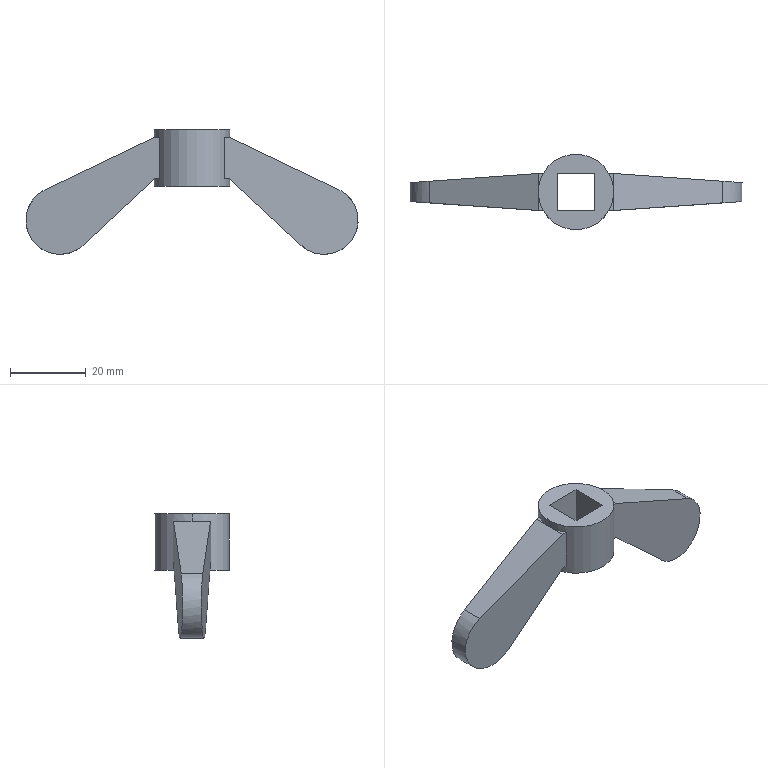Part | SolidWorks | features ICE 2, Extrusion 1, MirrorPattern 1 | 1 solid | 28 faces | box 88 x 20 x 33 mm | volume 11211 mm3 | plane 22 | cylinder 6 | commonest cylinder face diameters 18 x4 20 x2
STEP:
#1=CARTESIAN_POINT('',(35.,3.137,-25.5));
#2=VERTEX_POINT('',#1);
#3=CARTESIAN_POINT('',(28.863,3.571,-23.083));
#4=VERTEX_POINT('',#3);
#5=CARTESIAN_POINT('',(35.,3.137,-25.5));
#6=CARTESIAN_POINT('',(32.695,3.3,-25.5));
#7=CARTESIAN_POINT('',(30.55,3.452,-24.655));
#8=CARTESIAN_POINT('',(28.863,3.571,-23.083));
#9=(BOUNDED_CURVE()B_SPLINE_CURVE(3,(#5,#6,#7,#8),.UNSPECIFIED.,.F.,.T.)B_SPLINE_CURVE_WITH_KNOTS((4,4),(1.571,2.321),.UNSPECIFIED.)CURVE()GEOMETRIC_REPRESENTATION_ITEM()RATIONAL_B_SPLINE_CURVE((1.,0.9536,0.9536,1.))REPRESENTATION_ITEM(''));
#10=EDGE_CURVE('',#2,#4,#9,.T.);
#11=ORIENTED_EDGE('',*,*,#10,.F.);
#12=CARTESIAN_POINT('',(35.,-3.137,-25.5));
#13=VERTEX_POINT('',#12);
#14=CARTESIAN_POINT('',(35.,5.,-25.5));
#15=DIRECTION('',(0.,-1.,0.));
#16=VECTOR('',#15,1000.);
#17=LINE('',#14,#16);
#18=EDGE_CURVE('',#2,#13,#17,.T.);
#19=ORIENTED_EDGE('',*,*,#18,.T.);
#20=CARTESIAN_POINT('',(28.863,-3.571,-23.083));
#21=VERTEX_POINT('',#20);
#22=CARTESIAN_POINT('',(28.863,-3.571,-23.083));
#23=CARTESIAN_POINT('',(30.55,-3.452,-24.655));
#24=CARTESIAN_POINT('',(32.695,-3.3,-25.5));
#25=CARTESIAN_POINT('',(35.,-3.137,-25.5));
#26=(BOUNDED_CURVE()B_SPLINE_CURVE(3,(#22,#23,#24,#25),.UNSPECIFIED.,.F.,.T.)B_SPLINE_CURVE_WITH_KNOTS((4,4),(0.8205,1.571),.UNSPECIFIED.)CURVE()GEOMETRIC_REPRESENTATION_ITEM()RATIONAL_B_SPLINE_CURVE((1.,0.9536,0.9536,1.))REPRESENTATION_ITEM(''));
#27=EDGE_CURVE('',#21,#13,#26,.T.);
#28=ORIENTED_EDGE('',*,*,#27,.F.);
#29=CARTESIAN_POINT('',(28.863,5.,-23.083));
#30=DIRECTION('',(0.,-1.,0.));
#31=VECTOR('',#30,1000.);
#32=LINE('',#29,#31);
#33=EDGE_CURVE('',#4,#21,#32,.T.);
#34=ORIENTED_EDGE('',*,*,#33,.F.);
#35=EDGE_LOOP('',(#11,#19,#28,#34));
#36=FACE_OUTER_BOUND('',#35,.T.);
#37=CARTESIAN_POINT('',(35.,5.,-16.5));
#38=DIRECTION('',(0.,-1.,0.));
#39=DIRECTION('',(0.,0.,-1.));
#40=AXIS2_PLACEMENT_3D('',#37,#38,#39);
#41=CYLINDRICAL_SURFACE('',#40,9.);
#42=ADVANCED_FACE('',(#36),#41,.T.);
#43=CARTESIAN_POINT('',(10.,0.,7.5));
#44=VERTEX_POINT('',#43);
#45=CARTESIAN_POINT('',(-10.,0.,7.5));
#46=VERTEX_POINT('',#45);
#47=CARTESIAN_POINT('',(0.,0.,7.5));
#48=DIRECTION('',(0.,0.,1.));
#49=DIRECTION('',(1.,0.,0.));
#50=AXIS2_PLACEMENT_3D('',#47,#48,#49);
#51=CIRCLE('',#50,10.);
#52=EDGE_CURVE('',#44,#46,#51,.T.);
#53=ORIENTED_EDGE('',*,*,#52,.F.);
#54=CARTESIAN_POINT('',(10.,0.,5.5));
#55=VERTEX_POINT('',#54);
#56=CARTESIAN_POINT('',(10.,0.,7.5));
#57=DIRECTION('',(0.,0.,-1.));
#58=VECTOR('',#57,1000.);
#59=LINE('',#56,#58);
#60=EDGE_CURVE('',#44,#55,#59,.T.);
#61=ORIENTED_EDGE('',*,*,#60,.T.);
#62=CARTESIAN_POINT('',(8.66,5.,5.5));
#63=VERTEX_POINT('',#62);
#64=CARTESIAN_POINT('',(0.,0.,5.5));
#65=DIRECTION('',(0.,0.,-1.));
#66=DIRECTION('',(-1.,0.,0.));
#67=AXIS2_PLACEMENT_3D('',#64,#65,#66);
#68=CIRCLE('',#67,10.);
#69=EDGE_CURVE('',#63,#55,#68,.T.);
#70=ORIENTED_EDGE('',*,*,#69,.F.);
#71=CARTESIAN_POINT('',(8.66,5.,-5.5));
#72=VERTEX_POINT('',#71);
#73=CARTESIAN_POINT('',(8.66,5.,7.5));
#74=DIRECTION('',(0.,0.,-1.));
#75=VECTOR('',#74,1000.);
#76=LINE('',#73,#75);
#77=EDGE_CURVE('',#63,#72,#76,.T.);
#78=ORIENTED_EDGE('',*,*,#77,.T.);
#79=CARTESIAN_POINT('',(10.,0.,-5.5));
#80=VERTEX_POINT('',#79);
#81=CARTESIAN_POINT('',(0.,0.,-5.5));
#82=DIRECTION('',(0.,0.,1.));
#83=DIRECTION('',(1.,0.,0.));
#84=AXIS2_PLACEMENT_3D('',#81,#82,#83);
#85=CIRCLE('',#84,10.);
#86=EDGE_CURVE('',#80,#72,#85,.T.);
#87=ORIENTED_EDGE('',*,*,#86,.F.);
#88=CARTESIAN_POINT('',(10.,0.,-7.5));
#89=VERTEX_POINT('',#88);
#90=CARTESIAN_POINT('',(10.,0.,7.5));
#91=DIRECTION('',(0.,0.,-1.));
#92=VECTOR('',#91,1000.);
#93=LINE('',#90,#92);
#94=EDGE_CURVE('',#80,#89,#93,.T.);
#95=ORIENTED_EDGE('',*,*,#94,.T.);
#96=CARTESIAN_POINT('',(-10.,0.,-7.5));
#97=VERTEX_POINT('',#96);
#98=CARTESIAN_POINT('',(0.,0.,-7.5));
#99=DIRECTION('',(0.,0.,1.));
#100=DIRECTION('',(1.,0.,0.));
#101=AXIS2_PLACEMENT_3D('',#98,#99,#100);
#102=CIRCLE('',#101,10.);
#103=EDGE_CURVE('',#89,#97,#102,.T.);
#104=ORIENTED_EDGE('',*,*,#103,.T.);
#105=CARTESIAN_POINT('',(-10.,0.,-5.5));
#106=VERTEX_POINT('',#105);
#107=CARTESIAN_POINT('',(-10.,0.,7.5));
#108=DIRECTION('',(0.,0.,-1.));
#109=VECTOR('',#108,1000.);
#110=LINE('',#107,#109);
#111=EDGE_CURVE('',#106,#97,#110,.T.);
#112=ORIENTED_EDGE('',*,*,#111,.F.);
#113=CARTESIAN_POINT('',(-8.66,5.,-5.5));
#114=VERTEX_POINT('',#113);
#115=CARTESIAN_POINT('',(0.,0.,-5.5));
#116=DIRECTION('',(0.,0.,-1.));
#117=DIRECTION('',(-1.,0.,0.));
#118=AXIS2_PLACEMENT_3D('',#115,#116,#117);
#119=CIRCLE('',#118,10.);
#120=EDGE_CURVE('',#106,#114,#119,.T.);
#121=ORIENTED_EDGE('',*,*,#120,.T.);
#122=CARTESIAN_POINT('',(-8.66,5.,5.5));
#123=VERTEX_POINT('',#122);
#124=CARTESIAN_POINT('',(-8.66,5.,7.5));
#125=DIRECTION('',(0.,0.,1.));
#126=VECTOR('',#125,1000.);
#127=LINE('',#124,#126);
#128=EDGE_CURVE('',#114,#123,#127,.T.);
#129=ORIENTED_EDGE('',*,*,#128,.T.);
#130=CARTESIAN_POINT('',(-10.,0.,5.5));
#131=VERTEX_POINT('',#130);
#132=CARTESIAN_POINT('',(0.,0.,5.5));
#133=DIRECTION('',(0.,0.,1.));
#134=DIRECTION('',(1.,0.,0.));
#135=AXIS2_PLACEMENT_3D('',#132,#133,#134);
#136=CIRCLE('',#135,10.);
#137=EDGE_CURVE('',#123,#131,#136,.T.);
#138=ORIENTED_EDGE('',*,*,#137,.T.);
#139=CARTESIAN_POINT('',(-10.,0.,7.5));
#140=DIRECTION('',(0.,0.,-1.));
#141=VECTOR('',#140,1000.);
#142=LINE('',#139,#141);
#143=EDGE_CURVE('',#46,#131,#142,.T.);
#144=ORIENTED_EDGE('',*,*,#143,.F.);
#145=EDGE_LOOP('',(#53,#61,#70,#78,#87,#95,#104,#112,#121,#129,#138,#144));
#146=FACE_OUTER_BOUND('',#145,.T.);
#147=CARTESIAN_POINT('',(0.,0.,7.5));
#148=DIRECTION('',(0.,0.,-1.));
#149=DIRECTION('',(-1.,0.,0.));
#150=AXIS2_PLACEMENT_3D('',#147,#148,#149);
#151=CYLINDRICAL_SURFACE('',#150,10.);
#152=ADVANCED_FACE('',(#146),#151,.T.);
#153=CARTESIAN_POINT('',(-35.,3.137,-25.5));
#154=VERTEX_POINT('',#153);
#155=CARTESIAN_POINT('',(-38.898,2.861,-8.388));
#156=VERTEX_POINT('',#155);
#157=CARTESIAN_POINT('',(-35.,3.137,-25.5));
#158=CARTESIAN_POINT('',(-47.152,2.277,-25.5));
#159=CARTESIAN_POINT('',(-49.851,2.086,-13.652));
#160=CARTESIAN_POINT('',(-38.898,2.861,-8.388));
#161=(BOUNDED_CURVE()B_SPLINE_CURVE(3,(#157,#158,#159,#160),.UNSPECIFIED.,.F.,.T.)B_SPLINE_CURVE_WITH_KNOTS((4,4),(4.712,7.406),.UNSPECIFIED.)CURVE()GEOMETRIC_REPRESENTATION_ITEM()RATIONAL_B_SPLINE_CURVE((1.,0.4814,0.4814,1.))REPRESENTATION_ITEM(''));
#162=EDGE_CURVE('',#154,#156,#161,.T.);
#163=ORIENTED_EDGE('',*,*,#162,.F.);
#164=CARTESIAN_POINT('',(-35.,-3.137,-25.5));
#165=VERTEX_POINT('',#164);
#166=CARTESIAN_POINT('',(-35.,5.,-25.5));
#167=DIRECTION('',(0.,-1.,0.));
#168=VECTOR('',#167,1000.);
#169=LINE('',#166,#168);
#170=EDGE_CURVE('',#154,#165,#169,.T.);
#171=ORIENTED_EDGE('',*,*,#170,.T.);
#172=CARTESIAN_POINT('',(-38.898,-2.861,-8.388));
#173=VERTEX_POINT('',#172);
#174=CARTESIAN_POINT('',(-38.898,-2.861,-8.388));
#175=CARTESIAN_POINT('',(-49.851,-2.086,-13.652));
#176=CARTESIAN_POINT('',(-47.152,-2.277,-25.5));
#177=CARTESIAN_POINT('',(-35.,-3.137,-25.5));
#178=(BOUNDED_CURVE()B_SPLINE_CURVE(3,(#174,#175,#176,#177),.UNSPECIFIED.,.F.,.T.)B_SPLINE_CURVE_WITH_KNOTS((4,4),(2.019,4.712),.UNSPECIFIED.)CURVE()GEOMETRIC_REPRESENTATION_ITEM()RATIONAL_B_SPLINE_CURVE((1.,0.4814,0.4814,1.))REPRESENTATION_ITEM(''));
#179=EDGE_CURVE('',#173,#165,#178,.T.);
#180=ORIENTED_EDGE('',*,*,#179,.F.);
#181=CARTESIAN_POINT('',(-38.898,5.,-8.388));
#182=DIRECTION('',(0.,-1.,0.));
#183=VECTOR('',#182,1000.);
#184=LINE('',#181,#183);
#185=EDGE_CURVE('',#156,#173,#184,.T.);
#186=ORIENTED_EDGE('',*,*,#185,.F.);
#187=EDGE_LOOP('',(#163,#171,#180,#186));
#188=FACE_OUTER_BOUND('',#187,.T.);
#189=CARTESIAN_POINT('',(-35.,5.,-16.5));
#190=DIRECTION('',(0.,-1.,0.));
#191=DIRECTION('',(0.,0.,-1.));
#192=AXIS2_PLACEMENT_3D('',#189,#190,#191);
#193=CYLINDRICAL_SURFACE('',#192,9.);
#194=ADVANCED_FACE('',(#188),#193,.T.);
#195=CARTESIAN_POINT('',(-10.,-4.905,-5.5));
#196=VERTEX_POINT('',#195);
#197=CARTESIAN_POINT('',(-10.,5.,-5.5));
#198=DIRECTION('',(0.,-1.,0.));
#199=VECTOR('',#198,1000.);
#200=LINE('',#197,#199);
#201=EDGE_CURVE('',#106,#196,#200,.T.);
#202=ORIENTED_EDGE('',*,*,#201,.T.);
#203=CARTESIAN_POINT('',(-28.863,-3.571,-23.083));
#204=VERTEX_POINT('',#203);
#205=CARTESIAN_POINT('',(-2.302,-5.45,1.676));
#206=DIRECTION('',(-0.7305,0.05168,-0.6809));
#207=VECTOR('',#206,1000.);
#208=LINE('',#205,#207);
#209=EDGE_CURVE('',#196,#204,#208,.T.);
#210=ORIENTED_EDGE('',*,*,#209,.T.);
#211=CARTESIAN_POINT('',(-28.863,3.571,-23.083));
#212=VERTEX_POINT('',#211);
#213=CARTESIAN_POINT('',(-28.863,5.,-23.083));
#214=DIRECTION('',(0.,-1.,0.));
#215=VECTOR('',#214,1000.);
#216=LINE('',#213,#215);
#217=EDGE_CURVE('',#212,#204,#216,.T.);
#218=ORIENTED_EDGE('',*,*,#217,.F.);
#219=CARTESIAN_POINT('',(-10.,4.905,-5.5));
#220=VERTEX_POINT('',#219);
#221=CARTESIAN_POINT('',(-1.924,5.477,2.028));
#222=DIRECTION('',(0.7305,0.05168,0.6809));
#223=VECTOR('',#222,1000.);
#224=LINE('',#221,#223);
#225=EDGE_CURVE('',#212,#220,#224,.T.);
#226=ORIENTED_EDGE('',*,*,#225,.T.);
#227=CARTESIAN_POINT('',(-10.,5.,-5.5));
#228=DIRECTION('',(0.,-1.,0.));
#229=VECTOR('',#228,1000.);
#230=LINE('',#227,#229);
#231=EDGE_CURVE('',#220,#106,#230,.T.);
#232=ORIENTED_EDGE('',*,*,#231,.T.);
#233=EDGE_LOOP('',(#202,#210,#218,#226,#232));
#234=FACE_OUTER_BOUND('',#233,.T.);
#235=CARTESIAN_POINT('',(-1.906,5.,2.045));
#236=DIRECTION('',(0.6819,0.,-0.7315));
#237=DIRECTION('',(-0.7315,0.,-0.6819));
#238=AXIS2_PLACEMENT_3D('',#235,#236,#237);
#239=PLANE('',#238);
#240=ADVANCED_FACE('',(#234),#239,.T.);
#241=ORIENTED_EDGE('',*,*,#170,.F.);
#242=CARTESIAN_POINT('',(-28.863,3.571,-23.083));
#243=CARTESIAN_POINT('',(-30.55,3.452,-24.655));
#244=CARTESIAN_POINT('',(-32.695,3.3,-25.5));
#245=CARTESIAN_POINT('',(-35.,3.137,-25.5));
#246=(BOUNDED_CURVE()B_SPLINE_CURVE(3,(#242,#243,#244,#245),.UNSPECIFIED.,.F.,.T.)B_SPLINE_CURVE_WITH_KNOTS((4,4),(3.962,4.712),.UNSPECIFIED.)CURVE()GEOMETRIC_REPRESENTATION_ITEM()RATIONAL_B_SPLINE_CURVE((1.,0.9536,0.9536,1.))REPRESENTATION_ITEM(''));
#247=EDGE_CURVE('',#212,#154,#246,.T.);
#248=ORIENTED_EDGE('',*,*,#247,.F.);
#249=ORIENTED_EDGE('',*,*,#217,.T.);
#250=CARTESIAN_POINT('',(-35.,-3.137,-25.5));
#251=CARTESIAN_POINT('',(-32.695,-3.3,-25.5));
#252=CARTESIAN_POINT('',(-30.55,-3.452,-24.655));
#253=CARTESIAN_POINT('',(-28.863,-3.571,-23.083));
#254=(BOUNDED_CURVE()B_SPLINE_CURVE(3,(#250,#251,#252,#253),.UNSPECIFIED.,.F.,.F.)B_SPLINE_CURVE_WITH_KNOTS((4,4),(4.712,5.463),.UNSPECIFIED.)CURVE()GEOMETRIC_REPRESENTATION_ITEM()RATIONAL_B_SPLINE_CURVE((1.,0.9536,0.9536,1.))REPRESENTATION_ITEM(''));
#255=EDGE_CURVE('',#165,#204,#254,.T.);
#256=ORIENTED_EDGE('',*,*,#255,.F.);
#257=EDGE_LOOP('',(#241,#248,#249,#256));
#258=FACE_OUTER_BOUND('',#257,.T.);
#259=CARTESIAN_POINT('',(-35.,5.,-16.5));
#260=DIRECTION('',(0.,-1.,0.));
#261=DIRECTION('',(0.,0.,-1.));
#262=AXIS2_PLACEMENT_3D('',#259,#260,#261);
#263=CYLINDRICAL_SURFACE('',#262,9.);
#264=ADVANCED_FACE('',(#258),#263,.T.);
#265=CARTESIAN_POINT('',(-10.,-4.905,5.5));
#266=VERTEX_POINT('',#265);
#267=CARTESIAN_POINT('',(-4.615,-5.286,8.088));
#268=DIRECTION('',(-0.8995,0.06363,-0.4323));
#269=VECTOR('',#268,1000.);
#270=LINE('',#267,#269);
#271=EDGE_CURVE('',#266,#173,#270,.T.);
#272=ORIENTED_EDGE('',*,*,#271,.F.);
#273=CARTESIAN_POINT('',(-10.,5.,5.5));
#274=DIRECTION('',(0.,-1.,0.));
#275=VECTOR('',#274,1000.);
#276=LINE('',#273,#275);
#277=EDGE_CURVE('',#131,#266,#276,.T.);
#278=ORIENTED_EDGE('',*,*,#277,.F.);
#279=CARTESIAN_POINT('',(-10.,4.905,5.5));
#280=VERTEX_POINT('',#279);
#281=CARTESIAN_POINT('',(-10.,5.,5.5));
#282=DIRECTION('',(0.,-1.,0.));
#283=VECTOR('',#282,1000.);
#284=LINE('',#281,#283);
#285=EDGE_CURVE('',#280,#131,#284,.T.);
#286=ORIENTED_EDGE('',*,*,#285,.F.);
#287=CARTESIAN_POINT('',(-4.042,5.327,8.363));
#288=DIRECTION('',(0.8995,0.06363,0.4323));
#289=VECTOR('',#288,1000.);
#290=LINE('',#287,#289);
#291=EDGE_CURVE('',#156,#280,#290,.T.);
#292=ORIENTED_EDGE('',*,*,#291,.F.);
#293=ORIENTED_EDGE('',*,*,#185,.T.);
#294=EDGE_LOOP('',(#272,#278,#286,#292,#293));
#295=FACE_OUTER_BOUND('',#294,.T.);
#296=CARTESIAN_POINT('',(-4.024,5.,8.372));
#297=DIRECTION('',(0.4332,0.,-0.9013));
#298=DIRECTION('',(-0.9013,0.,-0.4332));
#299=AXIS2_PLACEMENT_3D('',#296,#297,#298);
#300=PLANE('',#299);
#301=ADVANCED_FACE('',(#295),#300,.F.);
#302=ORIENTED_EDGE('',*,*,#277,.T.);
#303=CARTESIAN_POINT('',(-8.66,-5.,5.5));
#304=VERTEX_POINT('',#303);
#305=CARTESIAN_POINT('',(-0.747,-5.56,5.5));
#306=DIRECTION('',(0.9975,-0.07057,0.));
#307=VECTOR('',#306,1000.);
#308=LINE('',#305,#307);
#309=EDGE_CURVE('',#266,#304,#308,.T.);
#310=ORIENTED_EDGE('',*,*,#309,.T.);
#311=CARTESIAN_POINT('',(0.,0.,5.5));
#312=DIRECTION('',(0.,0.,1.));
#313=DIRECTION('',(1.,0.,0.));
#314=AXIS2_PLACEMENT_3D('',#311,#312,#313);
#315=CIRCLE('',#314,10.);
#316=EDGE_CURVE('',#131,#304,#315,.T.);
#317=ORIENTED_EDGE('',*,*,#316,.F.);
#318=EDGE_LOOP('',(#302,#310,#317));
#319=FACE_OUTER_BOUND('',#318,.T.);
#320=CARTESIAN_POINT('',(0.,5.,5.5));
#321=DIRECTION('',(0.,0.,1.));
#322=DIRECTION('',(1.,0.,0.));
#323=AXIS2_PLACEMENT_3D('',#320,#321,#322);
#324=PLANE('',#323);
#325=ADVANCED_FACE('',(#319),#324,.T.);
#326=CARTESIAN_POINT('',(-8.66,-5.,-5.5));
#327=VERTEX_POINT('',#326);
#328=CARTESIAN_POINT('',(0.,0.,-5.5));
#329=DIRECTION('',(0.,0.,-1.));
#330=DIRECTION('',(-1.,0.,0.));
#331=AXIS2_PLACEMENT_3D('',#328,#329,#330);
#332=CIRCLE('',#331,10.);
#333=EDGE_CURVE('',#327,#106,#332,.T.);
#334=ORIENTED_EDGE('',*,*,#333,.F.);
#335=CARTESIAN_POINT('',(-0.747,-5.56,-5.5));
#336=DIRECTION('',(-0.9975,0.07057,0.));
#337=VECTOR('',#336,1000.);
#338=LINE('',#335,#337);
#339=EDGE_CURVE('',#327,#196,#338,.T.);
#340=ORIENTED_EDGE('',*,*,#339,.T.);
#341=ORIENTED_EDGE('',*,*,#201,.F.);
#342=EDGE_LOOP('',(#334,#340,#341));
#343=FACE_OUTER_BOUND('',#342,.T.);
#344=CARTESIAN_POINT('',(0.,5.,-5.5));
#345=DIRECTION('',(0.,0.,-1.));
#346=DIRECTION('',(-1.,0.,0.));
#347=AXIS2_PLACEMENT_3D('',#344,#345,#346);
#348=PLANE('',#347);
#349=ADVANCED_FACE('',(#343),#348,.T.);
#350=ORIENTED_EDGE('',*,*,#137,.F.);
#351=CARTESIAN_POINT('',(-0.04312,5.61,5.5));
#352=DIRECTION('',(-0.9975,-0.07057,0.));
#353=VECTOR('',#352,1000.);
#354=LINE('',#351,#353);
#355=EDGE_CURVE('',#123,#280,#354,.T.);
#356=ORIENTED_EDGE('',*,*,#355,.T.);
#357=ORIENTED_EDGE('',*,*,#285,.T.);
#358=EDGE_LOOP('',(#350,#356,#357));
#359=FACE_OUTER_BOUND('',#358,.T.);
#360=CARTESIAN_POINT('',(0.,5.,5.5));
#361=DIRECTION('',(0.,0.,1.));
#362=DIRECTION('',(1.,0.,0.));
#363=AXIS2_PLACEMENT_3D('',#360,#361,#362);
#364=PLANE('',#363);
#365=ADVANCED_FACE('',(#359),#364,.T.);
#366=ORIENTED_EDGE('',*,*,#231,.F.);
#367=CARTESIAN_POINT('',(-0.04312,5.61,-5.5));
#368=DIRECTION('',(0.9975,0.07057,0.));
#369=VECTOR('',#368,1000.);
#370=LINE('',#367,#369);
#371=EDGE_CURVE('',#220,#114,#370,.T.);
#372=ORIENTED_EDGE('',*,*,#371,.T.);
#373=ORIENTED_EDGE('',*,*,#120,.F.);
#374=EDGE_LOOP('',(#366,#372,#373));
#375=FACE_OUTER_BOUND('',#374,.T.);
#376=CARTESIAN_POINT('',(0.,5.,-5.5));
#377=DIRECTION('',(0.,0.,-1.));
#378=DIRECTION('',(-1.,0.,0.));
#379=AXIS2_PLACEMENT_3D('',#376,#377,#378);
#380=PLANE('',#379);
#381=ADVANCED_FACE('',(#375),#380,.T.);
#382=CARTESIAN_POINT('',(0.,0.,7.5));
#383=DIRECTION('',(0.,0.,1.));
#384=DIRECTION('',(1.,0.,0.));
#385=AXIS2_PLACEMENT_3D('',#382,#383,#384);
#386=CIRCLE('',#385,10.);
#387=EDGE_CURVE('',#46,#44,#386,.T.);
#388=ORIENTED_EDGE('',*,*,#387,.T.);
#389=ORIENTED_EDGE('',*,*,#52,.T.);
#390=EDGE_LOOP('',(#388,#389));
#391=FACE_OUTER_BOUND('',#390,.T.);
#392=CARTESIAN_POINT('',(5.,5.,7.5));
#393=VERTEX_POINT('',#392);
#394=CARTESIAN_POINT('',(-5.,5.,7.5));
#395=VERTEX_POINT('',#394);
#396=CARTESIAN_POINT('',(-5.,5.,7.5));
#397=DIRECTION('',(-1.,0.,0.));
#398=VECTOR('',#397,1000.);
#399=LINE('',#396,#398);
#400=EDGE_CURVE('',#393,#395,#399,.T.);
#401=ORIENTED_EDGE('',*,*,#400,.F.);
#402=CARTESIAN_POINT('',(5.,-5.,7.5));
#403=VERTEX_POINT('',#402);
#404=CARTESIAN_POINT('',(5.,-5.,7.5));
#405=DIRECTION('',(0.,1.,0.));
#406=VECTOR('',#405,1000.);
#407=LINE('',#404,#406);
#408=EDGE_CURVE('',#403,#393,#407,.T.);
#409=ORIENTED_EDGE('',*,*,#408,.F.);
#410=CARTESIAN_POINT('',(-5.,-5.,7.5));
#411=VERTEX_POINT('',#410);
#412=CARTESIAN_POINT('',(-5.,-5.,7.5));
#413=DIRECTION('',(1.,0.,0.));
#414=VECTOR('',#413,1000.);
#415=LINE('',#412,#414);
#416=EDGE_CURVE('',#411,#403,#415,.T.);
#417=ORIENTED_EDGE('',*,*,#416,.F.);
#418=CARTESIAN_POINT('',(-5.,-5.,7.5));
#419=DIRECTION('',(0.,-1.,0.));
#420=VECTOR('',#419,1000.);
#421=LINE('',#418,#420);
#422=EDGE_CURVE('',#395,#411,#421,.T.);
#423=ORIENTED_EDGE('',*,*,#422,.F.);
#424=EDGE_LOOP('',(#401,#409,#417,#423));
#425=FACE_BOUND('',#424,.T.);
#426=CARTESIAN_POINT('',(0.,0.,7.5));
#427=DIRECTION('',(0.,0.,1.));
#428=DIRECTION('',(1.,0.,0.));
#429=AXIS2_PLACEMENT_3D('',#426,#427,#428);
#430=PLANE('',#429);
#431=ADVANCED_FACE('',(#391,#425),#430,.T.);
#432=CARTESIAN_POINT('',(0.,0.,-7.5));
#433=DIRECTION('',(0.,0.,1.));
#434=DIRECTION('',(1.,0.,0.));
#435=AXIS2_PLACEMENT_3D('',#432,#433,#434);
#436=CIRCLE('',#435,10.);
#437=EDGE_CURVE('',#97,#89,#436,.T.);
#438=ORIENTED_EDGE('',*,*,#437,.F.);
#439=ORIENTED_EDGE('',*,*,#103,.F.);
#440=EDGE_LOOP('',(#438,#439));
#441=FACE_OUTER_BOUND('',#440,.T.);
#442=CARTESIAN_POINT('',(5.,-5.,-7.5));
#443=VERTEX_POINT('',#442);
#444=CARTESIAN_POINT('',(5.,5.,-7.5));
#445=VERTEX_POINT('',#444);
#446=CARTESIAN_POINT('',(5.,-5.,-7.5));
#447=DIRECTION('',(0.,1.,0.));
#448=VECTOR('',#447,1000.);
#449=LINE('',#446,#448);
#450=EDGE_CURVE('',#443,#445,#449,.T.);
#451=ORIENTED_EDGE('',*,*,#450,.T.);
#452=CARTESIAN_POINT('',(-5.,5.,-7.5));
#453=VERTEX_POINT('',#452);
#454=CARTESIAN_POINT('',(-5.,5.,-7.5));
#455=DIRECTION('',(-1.,0.,0.));
#456=VECTOR('',#455,1000.);
#457=LINE('',#454,#456);
#458=EDGE_CURVE('',#445,#453,#457,.T.);
#459=ORIENTED_EDGE('',*,*,#458,.T.);
#460=CARTESIAN_POINT('',(-5.,-5.,-7.5));
#461=VERTEX_POINT('',#460);
#462=CARTESIAN_POINT('',(-5.,-5.,-7.5));
#463=DIRECTION('',(0.,-1.,0.));
#464=VECTOR('',#463,1000.);
#465=LINE('',#462,#464);
#466=EDGE_CURVE('',#453,#461,#465,.T.);
#467=ORIENTED_EDGE('',*,*,#466,.T.);
#468=CARTESIAN_POINT('',(-5.,-5.,-7.5));
#469=DIRECTION('',(1.,0.,0.));
#470=VECTOR('',#469,1000.);
#471=LINE('',#468,#470);
#472=EDGE_CURVE('',#461,#443,#471,.T.);
#473=ORIENTED_EDGE('',*,*,#472,.T.);
#474=EDGE_LOOP('',(#451,#459,#467,#473));
#475=FACE_BOUND('',#474,.T.);
#476=CARTESIAN_POINT('',(0.,0.,-7.5));
#477=DIRECTION('',(0.,0.,1.));
#478=DIRECTION('',(1.,0.,0.));
#479=AXIS2_PLACEMENT_3D('',#476,#477,#478);
#480=PLANE('',#479);
#481=ADVANCED_FACE('',(#441,#475),#480,.F.);
#482=ORIENTED_EDGE('',*,*,#60,.F.);
#483=ORIENTED_EDGE('',*,*,#387,.F.);
#484=ORIENTED_EDGE('',*,*,#143,.T.);
#485=ORIENTED_EDGE('',*,*,#316,.T.);
#486=CARTESIAN_POINT('',(-8.66,-5.,7.5));
#487=DIRECTION('',(0.,0.,1.));
#488=VECTOR('',#487,1000.);
#489=LINE('',#486,#488);
#490=EDGE_CURVE('',#327,#304,#489,.T.);
#491=ORIENTED_EDGE('',*,*,#490,.F.);
#492=ORIENTED_EDGE('',*,*,#333,.T.);
#493=ORIENTED_EDGE('',*,*,#111,.T.);
#494=ORIENTED_EDGE('',*,*,#437,.T.);
#495=ORIENTED_EDGE('',*,*,#94,.F.);
#496=CARTESIAN_POINT('',(8.66,-5.,-5.5));
#497=VERTEX_POINT('',#496);
#498=CARTESIAN_POINT('',(0.,0.,-5.5));
#499=DIRECTION('',(0.,0.,1.));
#500=DIRECTION('',(1.,0.,0.));
#501=AXIS2_PLACEMENT_3D('',#498,#499,#500);
#502=CIRCLE('',#501,10.);
#503=EDGE_CURVE('',#497,#80,#502,.T.);
#504=ORIENTED_EDGE('',*,*,#503,.F.);
#505=CARTESIAN_POINT('',(8.66,-5.,5.5));
#506=VERTEX_POINT('',#505);
#507=CARTESIAN_POINT('',(8.66,-5.,7.5));
#508=DIRECTION('',(0.,0.,-1.));
#509=VECTOR('',#508,1000.);
#510=LINE('',#507,#509);
#511=EDGE_CURVE('',#506,#497,#510,.T.);
#512=ORIENTED_EDGE('',*,*,#511,.F.);
#513=CARTESIAN_POINT('',(0.,0.,5.5));
#514=DIRECTION('',(0.,0.,-1.));
#515=DIRECTION('',(-1.,0.,0.));
#516=AXIS2_PLACEMENT_3D('',#513,#514,#515);
#517=CIRCLE('',#516,10.);
#518=EDGE_CURVE('',#55,#506,#517,.T.);
#519=ORIENTED_EDGE('',*,*,#518,.F.);
#520=EDGE_LOOP('',(#482,#483,#484,#485,#491,#492,#493,#494,#495,#504,#512,#519));
#521=FACE_OUTER_BOUND('',#520,.T.);
#522=CARTESIAN_POINT('',(0.,0.,7.5));
#523=DIRECTION('',(0.,0.,-1.));
#524=DIRECTION('',(-1.,0.,0.));
#525=AXIS2_PLACEMENT_3D('',#522,#523,#524);
#526=CYLINDRICAL_SURFACE('',#525,10.);
#527=ADVANCED_FACE('',(#521),#526,.T.);
#528=ORIENTED_EDGE('',*,*,#450,.F.);
#529=CARTESIAN_POINT('',(5.,-5.,7.5));
#530=DIRECTION('',(0.,0.,-1.));
#531=VECTOR('',#530,1000.);
#532=LINE('',#529,#531);
#533=EDGE_CURVE('',#403,#443,#532,.T.);
#534=ORIENTED_EDGE('',*,*,#533,.F.);
#535=ORIENTED_EDGE('',*,*,#408,.T.);
#536=CARTESIAN_POINT('',(5.,5.,7.5));
#537=DIRECTION('',(0.,0.,-1.));
#538=VECTOR('',#537,1000.);
#539=LINE('',#536,#538);
#540=EDGE_CURVE('',#393,#445,#539,.T.);
#541=ORIENTED_EDGE('',*,*,#540,.T.);
#542=EDGE_LOOP('',(#528,#534,#535,#541));
#543=FACE_OUTER_BOUND('',#542,.T.);
#544=CARTESIAN_POINT('',(5.,-5.,7.5));
#545=DIRECTION('',(-1.,0.,0.));
#546=DIRECTION('',(0.,0.,1.));
#547=AXIS2_PLACEMENT_3D('',#544,#545,#546);
#548=PLANE('',#547);
#549=ADVANCED_FACE('',(#543),#548,.T.);
#550=ORIENTED_EDGE('',*,*,#458,.F.);
#551=ORIENTED_EDGE('',*,*,#540,.F.);
#552=ORIENTED_EDGE('',*,*,#400,.T.);
#553=CARTESIAN_POINT('',(-5.,5.,7.5));
#554=DIRECTION('',(0.,0.,-1.));
#555=VECTOR('',#554,1000.);
#556=LINE('',#553,#555);
#557=EDGE_CURVE('',#395,#453,#556,.T.);
#558=ORIENTED_EDGE('',*,*,#557,.T.);
#559=EDGE_LOOP('',(#550,#551,#552,#558));
#560=FACE_OUTER_BOUND('',#559,.T.);
#561=CARTESIAN_POINT('',(-5.,5.,7.5));
#562=DIRECTION('',(0.,-1.,0.));
#563=DIRECTION('',(0.,0.,-1.));
#564=AXIS2_PLACEMENT_3D('',#561,#562,#563);
#565=PLANE('',#564);
#566=ADVANCED_FACE('',(#560),#565,.T.);
#567=ORIENTED_EDGE('',*,*,#466,.F.);
#568=ORIENTED_EDGE('',*,*,#557,.F.);
#569=ORIENTED_EDGE('',*,*,#422,.T.);
#570=CARTESIAN_POINT('',(-5.,-5.,7.5));
#571=DIRECTION('',(0.,0.,-1.));
#572=VECTOR('',#571,1000.);
#573=LINE('',#570,#572);
#574=EDGE_CURVE('',#411,#461,#573,.T.);
#575=ORIENTED_EDGE('',*,*,#574,.T.);
#576=EDGE_LOOP('',(#567,#568,#569,#575));
#577=FACE_OUTER_BOUND('',#576,.T.);
#578=CARTESIAN_POINT('',(-5.,-5.,7.5));
#579=DIRECTION('',(1.,0.,0.));
#580=DIRECTION('',(0.,0.,-1.));
#581=AXIS2_PLACEMENT_3D('',#578,#579,#580);
#582=PLANE('',#581);
#583=ADVANCED_FACE('',(#577),#582,.T.);
#584=ORIENTED_EDGE('',*,*,#472,.F.);
#585=ORIENTED_EDGE('',*,*,#574,.F.);
#586=ORIENTED_EDGE('',*,*,#416,.T.);
#587=ORIENTED_EDGE('',*,*,#533,.T.);
#588=EDGE_LOOP('',(#584,#585,#586,#587));
#589=FACE_OUTER_BOUND('',#588,.T.);
#590=CARTESIAN_POINT('',(-5.,-5.,7.5));
#591=DIRECTION('',(0.,1.,0.));
#592=DIRECTION('',(0.,0.,1.));
#593=AXIS2_PLACEMENT_3D('',#590,#591,#592);
#594=PLANE('',#593);
#595=ADVANCED_FACE('',(#589),#594,.T.);
#596=ORIENTED_EDGE('',*,*,#225,.F.);
#597=ORIENTED_EDGE('',*,*,#247,.T.);
#598=ORIENTED_EDGE('',*,*,#162,.T.);
#599=ORIENTED_EDGE('',*,*,#291,.T.);
#600=ORIENTED_EDGE('',*,*,#355,.F.);
#601=ORIENTED_EDGE('',*,*,#128,.F.);
#602=ORIENTED_EDGE('',*,*,#371,.F.);
#603=EDGE_LOOP('',(#596,#597,#598,#599,#600,#601,#602));
#604=FACE_OUTER_BOUND('',#603,.T.);
#605=CARTESIAN_POINT('',(-0.3951,5.585,-38.));
#606=DIRECTION('',(-0.07057,0.9975,0.));
#607=DIRECTION('',(-0.9975,-0.07057,0.));
#608=AXIS2_PLACEMENT_3D('',#605,#606,#607);
#609=PLANE('',#608);
#610=ADVANCED_FACE('',(#604),#609,.T.);
#611=ORIENTED_EDGE('',*,*,#271,.T.);
#612=ORIENTED_EDGE('',*,*,#179,.T.);
#613=ORIENTED_EDGE('',*,*,#255,.T.);
#614=ORIENTED_EDGE('',*,*,#209,.F.);
#615=ORIENTED_EDGE('',*,*,#339,.F.);
#616=ORIENTED_EDGE('',*,*,#490,.T.);
#617=ORIENTED_EDGE('',*,*,#309,.F.);
#618=EDGE_LOOP('',(#611,#612,#613,#614,#615,#616,#617));
#619=FACE_OUTER_BOUND('',#618,.T.);
#620=CARTESIAN_POINT('',(-0.3951,-5.585,-38.));
#621=DIRECTION('',(-0.07057,-0.9975,0.));
#622=DIRECTION('',(0.9975,-0.07057,0.));
#623=AXIS2_PLACEMENT_3D('',#620,#621,#622);
#624=PLANE('',#623);
#625=ADVANCED_FACE('',(#619),#624,.T.);
#626=ORIENTED_EDGE('',*,*,#86,.T.);
#627=CARTESIAN_POINT('',(10.,4.905,-5.5));
#628=VERTEX_POINT('',#627);
#629=CARTESIAN_POINT('',(0.04312,5.61,-5.5));
#630=DIRECTION('',(0.9975,-0.07057,0.));
#631=VECTOR('',#630,1000.);
#632=LINE('',#629,#631);
#633=EDGE_CURVE('',#72,#628,#632,.T.);
#634=ORIENTED_EDGE('',*,*,#633,.T.);
#635=CARTESIAN_POINT('',(10.,5.,-5.5));
#636=DIRECTION('',(0.,-1.,0.));
#637=VECTOR('',#636,1000.);
#638=LINE('',#635,#637);
#639=EDGE_CURVE('',#628,#80,#638,.T.);
#640=ORIENTED_EDGE('',*,*,#639,.T.);
#641=EDGE_LOOP('',(#626,#634,#640));
#642=FACE_OUTER_BOUND('',#641,.T.);
#643=CARTESIAN_POINT('',(0.,5.,-5.5));
#644=DIRECTION('',(0.,0.,1.));
#645=DIRECTION('',(1.,0.,0.));
#646=AXIS2_PLACEMENT_3D('',#643,#644,#645);
#647=PLANE('',#646);
#648=ADVANCED_FACE('',(#642),#647,.F.);
#649=CARTESIAN_POINT('',(10.,-4.905,-5.5));
#650=VERTEX_POINT('',#649);
#651=CARTESIAN_POINT('',(10.,5.,-5.5));
#652=DIRECTION('',(0.,-1.,0.));
#653=VECTOR('',#652,1000.);
#654=LINE('',#651,#653);
#655=EDGE_CURVE('',#80,#650,#654,.T.);
#656=ORIENTED_EDGE('',*,*,#655,.T.);
#657=CARTESIAN_POINT('',(0.747,-5.56,-5.5));
#658=DIRECTION('',(-0.9975,-0.07057,0.));
#659=VECTOR('',#658,1000.);
#660=LINE('',#657,#659);
#661=EDGE_CURVE('',#650,#497,#660,.T.);
#662=ORIENTED_EDGE('',*,*,#661,.T.);
#663=ORIENTED_EDGE('',*,*,#503,.T.);
#664=EDGE_LOOP('',(#656,#662,#663));
#665=FACE_OUTER_BOUND('',#664,.T.);
#666=CARTESIAN_POINT('',(0.,5.,-5.5));
#667=DIRECTION('',(0.,0.,1.));
#668=DIRECTION('',(1.,0.,0.));
#669=AXIS2_PLACEMENT_3D('',#666,#667,#668);
#670=PLANE('',#669);
#671=ADVANCED_FACE('',(#665),#670,.F.);
#672=CARTESIAN_POINT('',(10.,4.905,5.5));
#673=VERTEX_POINT('',#672);
#674=CARTESIAN_POINT('',(10.,5.,5.5));
#675=DIRECTION('',(0.,-1.,0.));
#676=VECTOR('',#675,1000.);
#677=LINE('',#674,#676);
#678=EDGE_CURVE('',#673,#55,#677,.T.);
#679=ORIENTED_EDGE('',*,*,#678,.F.);
#680=CARTESIAN_POINT('',(0.04312,5.61,5.5));
#681=DIRECTION('',(-0.9975,0.07057,0.));
#682=VECTOR('',#681,1000.);
#683=LINE('',#680,#682);
#684=EDGE_CURVE('',#673,#63,#683,.T.);
#685=ORIENTED_EDGE('',*,*,#684,.T.);
#686=ORIENTED_EDGE('',*,*,#69,.T.);
#687=EDGE_LOOP('',(#679,#685,#686));
#688=FACE_OUTER_BOUND('',#687,.T.);
#689=CARTESIAN_POINT('',(0.,5.,5.5));
#690=DIRECTION('',(0.,0.,-1.));
#691=DIRECTION('',(-1.,0.,0.));
#692=AXIS2_PLACEMENT_3D('',#689,#690,#691);
#693=PLANE('',#692);
#694=ADVANCED_FACE('',(#688),#693,.F.);
#695=ORIENTED_EDGE('',*,*,#518,.T.);
#696=CARTESIAN_POINT('',(10.,-4.905,5.5));
#697=VERTEX_POINT('',#696);
#698=CARTESIAN_POINT('',(0.747,-5.56,5.5));
#699=DIRECTION('',(0.9975,0.07057,0.));
#700=VECTOR('',#699,1000.);
#701=LINE('',#698,#700);
#702=EDGE_CURVE('',#506,#697,#701,.T.);
#703=ORIENTED_EDGE('',*,*,#702,.T.);
#704=CARTESIAN_POINT('',(10.,5.,5.5));
#705=DIRECTION('',(0.,-1.,0.));
#706=VECTOR('',#705,1000.);
#707=LINE('',#704,#706);
#708=EDGE_CURVE('',#55,#697,#707,.T.);
#709=ORIENTED_EDGE('',*,*,#708,.F.);
#710=EDGE_LOOP('',(#695,#703,#709));
#711=FACE_OUTER_BOUND('',#710,.T.);
#712=CARTESIAN_POINT('',(0.,5.,5.5));
#713=DIRECTION('',(0.,0.,-1.));
#714=DIRECTION('',(-1.,0.,0.));
#715=AXIS2_PLACEMENT_3D('',#712,#713,#714);
#716=PLANE('',#715);
#717=ADVANCED_FACE('',(#711),#716,.F.);
#718=ORIENTED_EDGE('',*,*,#33,.T.);
#719=CARTESIAN_POINT('',(2.302,-5.45,1.676));
#720=DIRECTION('',(-0.7305,-0.05168,0.6809));
#721=VECTOR('',#720,1000.);
#722=LINE('',#719,#721);
#723=EDGE_CURVE('',#21,#650,#722,.T.);
#724=ORIENTED_EDGE('',*,*,#723,.T.);
#725=ORIENTED_EDGE('',*,*,#655,.F.);
#726=ORIENTED_EDGE('',*,*,#639,.F.);
#727=CARTESIAN_POINT('',(1.924,5.477,2.028));
#728=DIRECTION('',(0.7305,-0.05168,-0.6809));
#729=VECTOR('',#728,1000.);
#730=LINE('',#727,#729);
#731=EDGE_CURVE('',#628,#4,#730,.T.);
#732=ORIENTED_EDGE('',*,*,#731,.T.);
#733=EDGE_LOOP('',(#718,#724,#725,#726,#732));
#734=FACE_OUTER_BOUND('',#733,.T.);
#735=CARTESIAN_POINT('',(1.906,5.,2.045));
#736=DIRECTION('',(0.6819,0.,0.7315));
#737=DIRECTION('',(0.7315,0.,-0.6819));
#738=AXIS2_PLACEMENT_3D('',#735,#736,#737);
#739=PLANE('',#738);
#740=ADVANCED_FACE('',(#734),#739,.F.);
#741=CARTESIAN_POINT('',(38.898,-2.861,-8.388));
#742=VERTEX_POINT('',#741);
#743=CARTESIAN_POINT('',(4.615,-5.286,8.088));
#744=DIRECTION('',(-0.8995,-0.06363,0.4323));
#745=VECTOR('',#744,1000.);
#746=LINE('',#743,#745);
#747=EDGE_CURVE('',#742,#697,#746,.T.);
#748=ORIENTED_EDGE('',*,*,#747,.F.);
#749=CARTESIAN_POINT('',(38.898,2.861,-8.388));
#750=VERTEX_POINT('',#749);
#751=CARTESIAN_POINT('',(38.898,5.,-8.388));
#752=DIRECTION('',(0.,-1.,0.));
#753=VECTOR('',#752,1000.);
#754=LINE('',#751,#753);
#755=EDGE_CURVE('',#750,#742,#754,.T.);
#756=ORIENTED_EDGE('',*,*,#755,.F.);
#757=CARTESIAN_POINT('',(4.042,5.327,8.363));
#758=DIRECTION('',(0.8995,-0.06363,-0.4323));
#759=VECTOR('',#758,1000.);
#760=LINE('',#757,#759);
#761=EDGE_CURVE('',#673,#750,#760,.T.);
#762=ORIENTED_EDGE('',*,*,#761,.F.);
#763=ORIENTED_EDGE('',*,*,#678,.T.);
#764=ORIENTED_EDGE('',*,*,#708,.T.);
#765=EDGE_LOOP('',(#748,#756,#762,#763,#764));
#766=FACE_OUTER_BOUND('',#765,.T.);
#767=CARTESIAN_POINT('',(4.024,5.,8.372));
#768=DIRECTION('',(0.4332,0.,0.9013));
#769=DIRECTION('',(0.9013,0.,-0.4332));
#770=AXIS2_PLACEMENT_3D('',#767,#768,#769);
#771=PLANE('',#770);
#772=ADVANCED_FACE('',(#766),#771,.T.);
#773=ORIENTED_EDGE('',*,*,#18,.F.);
#774=CARTESIAN_POINT('',(38.898,2.861,-8.388));
#775=CARTESIAN_POINT('',(49.851,2.086,-13.652));
#776=CARTESIAN_POINT('',(47.152,2.277,-25.5));
#777=CARTESIAN_POINT('',(35.,3.137,-25.5));
#778=(BOUNDED_CURVE()B_SPLINE_CURVE(3,(#774,#775,#776,#777),.UNSPECIFIED.,.F.,.T.)B_SPLINE_CURVE_WITH_KNOTS((4,4),(5.16,7.854),.UNSPECIFIED.)CURVE()GEOMETRIC_REPRESENTATION_ITEM()RATIONAL_B_SPLINE_CURVE((1.,0.4814,0.4814,1.))REPRESENTATION_ITEM(''));
#779=EDGE_CURVE('',#750,#2,#778,.T.);
#780=ORIENTED_EDGE('',*,*,#779,.F.);
#781=ORIENTED_EDGE('',*,*,#755,.T.);
#782=CARTESIAN_POINT('',(35.,-3.137,-25.5));
#783=CARTESIAN_POINT('',(47.152,-2.277,-25.5));
#784=CARTESIAN_POINT('',(49.851,-2.086,-13.652));
#785=CARTESIAN_POINT('',(38.898,-2.861,-8.388));
#786=(BOUNDED_CURVE()B_SPLINE_CURVE(3,(#782,#783,#784,#785),.UNSPECIFIED.,.F.,.T.)B_SPLINE_CURVE_WITH_KNOTS((4,4),(1.571,4.264),.UNSPECIFIED.)CURVE()GEOMETRIC_REPRESENTATION_ITEM()RATIONAL_B_SPLINE_CURVE((1.,0.4814,0.4814,1.))REPRESENTATION_ITEM(''));
#787=EDGE_CURVE('',#13,#742,#786,.T.);
#788=ORIENTED_EDGE('',*,*,#787,.F.);
#789=EDGE_LOOP('',(#773,#780,#781,#788));
#790=FACE_OUTER_BOUND('',#789,.T.);
#791=CARTESIAN_POINT('',(35.,5.,-16.5));
#792=DIRECTION('',(0.,-1.,0.));
#793=DIRECTION('',(0.,0.,-1.));
#794=AXIS2_PLACEMENT_3D('',#791,#792,#793);
#795=CYLINDRICAL_SURFACE('',#794,9.);
#796=ADVANCED_FACE('',(#790),#795,.T.);
#797=ORIENTED_EDGE('',*,*,#77,.F.);
#798=ORIENTED_EDGE('',*,*,#684,.F.);
#799=ORIENTED_EDGE('',*,*,#761,.T.);
#800=ORIENTED_EDGE('',*,*,#779,.T.);
#801=ORIENTED_EDGE('',*,*,#10,.T.);
#802=ORIENTED_EDGE('',*,*,#731,.F.);
#803=ORIENTED_EDGE('',*,*,#633,.F.);
#804=EDGE_LOOP('',(#797,#798,#799,#800,#801,#802,#803));
#805=FACE_OUTER_BOUND('',#804,.T.);
#806=CARTESIAN_POINT('',(0.3951,5.585,-38.));
#807=DIRECTION('',(-0.07057,-0.9975,0.));
#808=DIRECTION('',(0.9975,-0.07057,0.));
#809=AXIS2_PLACEMENT_3D('',#806,#807,#808);
#810=PLANE('',#809);
#811=ADVANCED_FACE('',(#805),#810,.F.);
#812=ORIENTED_EDGE('',*,*,#723,.F.);
#813=ORIENTED_EDGE('',*,*,#27,.T.);
#814=ORIENTED_EDGE('',*,*,#787,.T.);
#815=ORIENTED_EDGE('',*,*,#747,.T.);
#816=ORIENTED_EDGE('',*,*,#702,.F.);
#817=ORIENTED_EDGE('',*,*,#511,.T.);
#818=ORIENTED_EDGE('',*,*,#661,.F.);
#819=EDGE_LOOP('',(#812,#813,#814,#815,#816,#817,#818));
#820=FACE_OUTER_BOUND('',#819,.T.);
#821=CARTESIAN_POINT('',(0.3951,-5.585,-38.));
#822=DIRECTION('',(-0.07057,0.9975,0.));
#823=DIRECTION('',(-0.9975,-0.07057,0.));
#824=AXIS2_PLACEMENT_3D('',#821,#822,#823);
#825=PLANE('',#824);
#826=ADVANCED_FACE('',(#820),#825,.F.);
#827=CLOSED_SHELL('',(#42,#152,#194,#240,#264,#301,#325,#349,#365,#381,#431,#481,#527,#549,#566,#583,#595,#610,#625,#648,#671,#694,#717,#740,#772,#796,#811,#826));
#828=MANIFOLD_SOLID_BREP('',#827);
#829=CARTESIAN_POINT('',(0.,0.,0.));
#830=DIRECTION('',(0.,0.,1.));
#831=DIRECTION('',(1.,0.,0.));
#832=AXIS2_PLACEMENT_3D('',#829,#830,#831);
#833=(LENGTH_UNIT()NAMED_UNIT(*)SI_UNIT(.MILLI.,.METRE.));
#834=UNCERTAINTY_MEASURE_WITH_UNIT(LENGTH_MEASURE(0.00001),#833,'','');
#835=(NAMED_UNIT(*)PLANE_ANGLE_UNIT()SI_UNIT($,.RADIAN.));
#836=(NAMED_UNIT(*)SI_UNIT($,.STERADIAN.)SOLID_ANGLE_UNIT());
#837=(GEOMETRIC_REPRESENTATION_CONTEXT(3)GLOBAL_UNCERTAINTY_ASSIGNED_CONTEXT((#834))GLOBAL_UNIT_ASSIGNED_CONTEXT((#833,#835,#836))REPRESENTATION_CONTEXT('',''));
#838=ADVANCED_BREP_SHAPE_REPRESENTATION('',(#828,#832),#837);